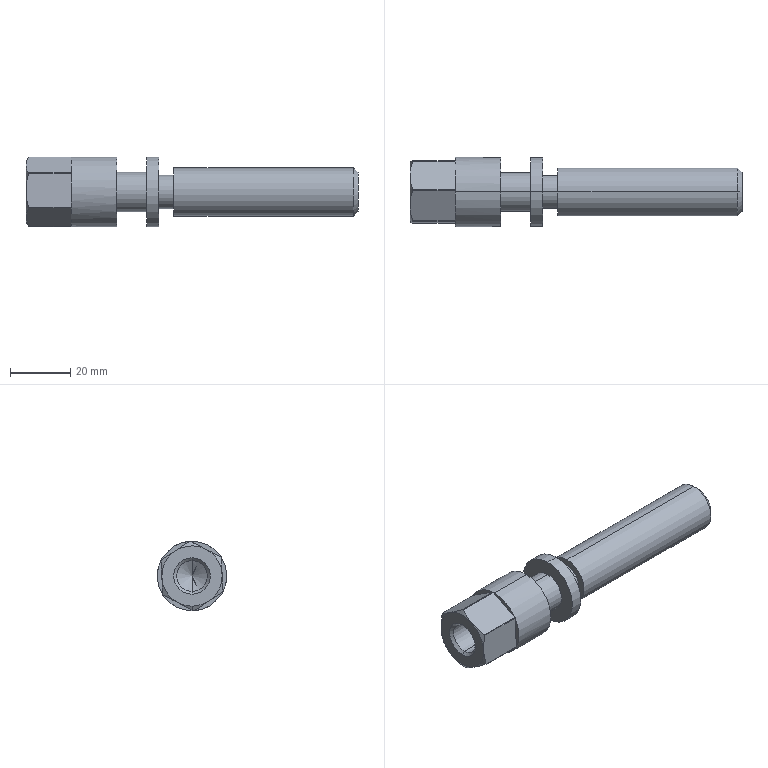Part | SolidWorks | features 3DProfileFeature 1, Chamfer 1, HoleWzd 1, ICE 1, Revolution 1 | 1 solid | 43 faces | box 110 x 23 x 23 mm | volume 25098 mm3 | plane 18 | cone 13 | cylinder 12 | commonest cylinder face diameters 23 x4 10.2 x2 11 x2 13 x2 16 x2
STEP:
#1=CARTESIAN_POINT('',(110.,0.,-6.5));
#2=VERTEX_POINT('',#1);
#3=CARTESIAN_POINT('',(110.,0.,6.5));
#4=VERTEX_POINT('',#3);
#5=CARTESIAN_POINT('',(110.,0.,0.));
#6=DIRECTION('',(1.,0.,0.));
#7=DIRECTION('',(0.,0.,1.));
#8=AXIS2_PLACEMENT_3D('',#5,#6,#7);
#9=CIRCLE('',#8,6.5);
#10=EDGE_CURVE('',#2,#4,#9,.T.);
#11=ORIENTED_EDGE('',*,*,#10,.F.);
#12=CARTESIAN_POINT('',(108.5,0.,-8.));
#13=VERTEX_POINT('',#12);
#14=CARTESIAN_POINT('',(108.5,0.,-8.));
#15=DIRECTION('',(-0.7071,0.,-0.7071));
#16=VECTOR('',#15,1000.);
#17=LINE('',#14,#16);
#18=EDGE_CURVE('',#2,#13,#17,.T.);
#19=ORIENTED_EDGE('',*,*,#18,.T.);
#20=CARTESIAN_POINT('',(108.5,0.,8.));
#21=VERTEX_POINT('',#20);
#22=CARTESIAN_POINT('',(108.5,0.,0.));
#23=DIRECTION('',(-1.,0.,0.));
#24=DIRECTION('',(0.,0.,1.));
#25=AXIS2_PLACEMENT_3D('',#22,#23,#24);
#26=CIRCLE('',#25,8.);
#27=EDGE_CURVE('',#21,#13,#26,.T.);
#28=ORIENTED_EDGE('',*,*,#27,.F.);
#29=CARTESIAN_POINT('',(108.5,0.,8.));
#30=DIRECTION('',(-0.7071,0.,0.7071));
#31=VECTOR('',#30,1000.);
#32=LINE('',#29,#31);
#33=EDGE_CURVE('',#4,#21,#32,.T.);
#34=ORIENTED_EDGE('',*,*,#33,.F.);
#35=EDGE_LOOP('',(#11,#19,#28,#34));
#36=FACE_OUTER_BOUND('',#35,.T.);
#37=CARTESIAN_POINT('',(108.5,0.,0.));
#38=DIRECTION('',(-1.,0.,0.));
#39=DIRECTION('',(0.,0.,1.));
#40=AXIS2_PLACEMENT_3D('',#37,#38,#39);
#41=CONICAL_SURFACE('',#40,8.,0.7854);
#42=ADVANCED_FACE('',(#36),#41,.T.);
#43=CARTESIAN_POINT('',(0.925,0.,-5.1));
#44=VERTEX_POINT('',#43);
#45=CARTESIAN_POINT('',(0.925,0.,5.1));
#46=VERTEX_POINT('',#45);
#47=CARTESIAN_POINT('',(0.925,0.,0.));
#48=DIRECTION('',(-1.,0.,0.));
#49=DIRECTION('',(0.,0.,1.));
#50=AXIS2_PLACEMENT_3D('',#47,#48,#49);
#51=CIRCLE('',#50,5.1);
#52=EDGE_CURVE('',#44,#46,#51,.T.);
#53=ORIENTED_EDGE('',*,*,#52,.F.);
#54=CARTESIAN_POINT('',(0.,0.,-6.025));
#55=VERTEX_POINT('',#54);
#56=CARTESIAN_POINT('',(0.,0.,-6.025));
#57=DIRECTION('',(-0.7071,0.,-0.7071));
#58=VECTOR('',#57,1000.);
#59=LINE('',#56,#58);
#60=EDGE_CURVE('',#44,#55,#59,.T.);
#61=ORIENTED_EDGE('',*,*,#60,.T.);
#62=CARTESIAN_POINT('',(0.,0.,6.025));
#63=VERTEX_POINT('',#62);
#64=CARTESIAN_POINT('',(0.,0.,0.));
#65=DIRECTION('',(-1.,0.,0.));
#66=DIRECTION('',(0.,0.,1.));
#67=AXIS2_PLACEMENT_3D('',#64,#65,#66);
#68=CIRCLE('',#67,6.025);
#69=EDGE_CURVE('',#55,#63,#68,.T.);
#70=ORIENTED_EDGE('',*,*,#69,.T.);
#71=CARTESIAN_POINT('',(0.,0.,6.025));
#72=DIRECTION('',(-0.7071,0.,0.7071));
#73=VECTOR('',#72,1000.);
#74=LINE('',#71,#73);
#75=EDGE_CURVE('',#46,#63,#74,.T.);
#76=ORIENTED_EDGE('',*,*,#75,.F.);
#77=EDGE_LOOP('',(#53,#61,#70,#76));
#78=FACE_OUTER_BOUND('',#77,.T.);
#79=CARTESIAN_POINT('',(0.,0.,0.));
#80=DIRECTION('',(-1.,0.,0.));
#81=DIRECTION('',(0.,0.,1.));
#82=AXIS2_PLACEMENT_3D('',#79,#80,#81);
#83=CONICAL_SURFACE('',#82,6.025,0.7854);
#84=ADVANCED_FACE('',(#78),#83,.F.);
#85=CARTESIAN_POINT('',(23.25,0.,-5.1));
#86=VERTEX_POINT('',#85);
#87=CARTESIAN_POINT('',(23.25,0.,5.1));
#88=VERTEX_POINT('',#87);
#89=CARTESIAN_POINT('',(23.25,0.,0.));
#90=DIRECTION('',(-1.,0.,0.));
#91=DIRECTION('',(0.,0.,1.));
#92=AXIS2_PLACEMENT_3D('',#89,#90,#91);
#93=CIRCLE('',#92,5.1);
#94=EDGE_CURVE('',#86,#88,#93,.T.);
#95=ORIENTED_EDGE('',*,*,#94,.F.);
#96=CARTESIAN_POINT('',(0.,0.,-5.1));
#97=DIRECTION('',(-1.,0.,0.));
#98=VECTOR('',#97,1000.);
#99=LINE('',#96,#98);
#100=EDGE_CURVE('',#86,#44,#99,.T.);
#101=ORIENTED_EDGE('',*,*,#100,.T.);
#102=ORIENTED_EDGE('',*,*,#52,.T.);
#103=CARTESIAN_POINT('',(0.,0.,5.1));
#104=DIRECTION('',(-1.,0.,0.));
#105=VECTOR('',#104,1000.);
#106=LINE('',#103,#105);
#107=EDGE_CURVE('',#88,#46,#106,.T.);
#108=ORIENTED_EDGE('',*,*,#107,.F.);
#109=EDGE_LOOP('',(#95,#101,#102,#108));
#110=FACE_OUTER_BOUND('',#109,.T.);
#111=CARTESIAN_POINT('',(0.,0.,0.));
#112=DIRECTION('',(-1.,0.,0.));
#113=DIRECTION('',(0.,0.,1.));
#114=AXIS2_PLACEMENT_3D('',#111,#112,#113);
#115=CYLINDRICAL_SURFACE('',#114,5.1);
#116=ADVANCED_FACE('',(#110),#115,.F.);
#117=CARTESIAN_POINT('',(26.314,0.,0.));
#118=VERTEX_POINT('',#117);
#119=CARTESIAN_POINT('',(23.25,0.,5.1));
#120=DIRECTION('',(-0.515,0.,0.8572));
#121=VECTOR('',#120,1000.);
#122=LINE('',#119,#121);
#123=EDGE_CURVE('',#118,#88,#122,.T.);
#124=ORIENTED_EDGE('',*,*,#123,.F.);
#125=CARTESIAN_POINT('',(23.25,0.,-5.1));
#126=DIRECTION('',(-0.515,0.,-0.8572));
#127=VECTOR('',#126,1000.);
#128=LINE('',#125,#127);
#129=EDGE_CURVE('',#118,#86,#128,.T.);
#130=ORIENTED_EDGE('',*,*,#129,.T.);
#131=ORIENTED_EDGE('',*,*,#94,.T.);
#132=EDGE_LOOP('',(#124,#130,#131));
#133=FACE_OUTER_BOUND('',#132,.T.);
#134=CARTESIAN_POINT('',(23.25,0.,0.));
#135=DIRECTION('',(-1.,0.,0.));
#136=DIRECTION('',(0.,0.,1.));
#137=AXIS2_PLACEMENT_3D('',#134,#135,#136);
#138=CONICAL_SURFACE('',#137,5.1,1.03);
#139=ADVANCED_FACE('',(#133),#138,.F.);
#140=ORIENTED_EDGE('',*,*,#27,.T.);
#141=CARTESIAN_POINT('',(49.,0.,-8.));
#142=VERTEX_POINT('',#141);
#143=CARTESIAN_POINT('',(0.,0.,-8.));
#144=DIRECTION('',(-1.,0.,0.));
#145=VECTOR('',#144,1000.);
#146=LINE('',#143,#145);
#147=EDGE_CURVE('',#13,#142,#146,.T.);
#148=ORIENTED_EDGE('',*,*,#147,.T.);
#149=CARTESIAN_POINT('',(49.,0.,8.));
#150=VERTEX_POINT('',#149);
#151=CARTESIAN_POINT('',(49.,0.,0.));
#152=DIRECTION('',(-1.,0.,0.));
#153=DIRECTION('',(0.,0.,1.));
#154=AXIS2_PLACEMENT_3D('',#151,#152,#153);
#155=CIRCLE('',#154,8.);
#156=EDGE_CURVE('',#150,#142,#155,.T.);
#157=ORIENTED_EDGE('',*,*,#156,.F.);
#158=CARTESIAN_POINT('',(0.,0.,8.));
#159=DIRECTION('',(-1.,0.,0.));
#160=VECTOR('',#159,1000.);
#161=LINE('',#158,#160);
#162=EDGE_CURVE('',#21,#150,#161,.T.);
#163=ORIENTED_EDGE('',*,*,#162,.F.);
#164=EDGE_LOOP('',(#140,#148,#157,#163));
#165=FACE_OUTER_BOUND('',#164,.T.);
#166=CARTESIAN_POINT('',(0.,0.,0.));
#167=DIRECTION('',(-1.,0.,0.));
#168=DIRECTION('',(0.,0.,1.));
#169=AXIS2_PLACEMENT_3D('',#166,#167,#168);
#170=CYLINDRICAL_SURFACE('',#169,8.);
#171=ADVANCED_FACE('',(#165),#170,.T.);
#172=CARTESIAN_POINT('',(49.,0.,5.5));
#173=VERTEX_POINT('',#172);
#174=CARTESIAN_POINT('',(49.,0.,-5.5));
#175=VERTEX_POINT('',#174);
#176=CARTESIAN_POINT('',(49.,0.,0.));
#177=DIRECTION('',(-1.,0.,0.));
#178=DIRECTION('',(0.,0.,1.));
#179=AXIS2_PLACEMENT_3D('',#176,#177,#178);
#180=CIRCLE('',#179,5.5);
#181=EDGE_CURVE('',#173,#175,#180,.T.);
#182=ORIENTED_EDGE('',*,*,#181,.T.);
#183=CARTESIAN_POINT('',(44.,0.,-5.5));
#184=VERTEX_POINT('',#183);
#185=CARTESIAN_POINT('',(0.,0.,-5.5));
#186=DIRECTION('',(-1.,0.,0.));
#187=VECTOR('',#186,1000.);
#188=LINE('',#185,#187);
#189=EDGE_CURVE('',#175,#184,#188,.T.);
#190=ORIENTED_EDGE('',*,*,#189,.T.);
#191=CARTESIAN_POINT('',(44.,0.,5.5));
#192=VERTEX_POINT('',#191);
#193=CARTESIAN_POINT('',(44.,0.,0.));
#194=DIRECTION('',(-1.,0.,0.));
#195=DIRECTION('',(0.,0.,1.));
#196=AXIS2_PLACEMENT_3D('',#193,#194,#195);
#197=CIRCLE('',#196,5.5);
#198=EDGE_CURVE('',#192,#184,#197,.T.);
#199=ORIENTED_EDGE('',*,*,#198,.F.);
#200=CARTESIAN_POINT('',(0.,0.,5.5));
#201=DIRECTION('',(-1.,0.,0.));
#202=VECTOR('',#201,1000.);
#203=LINE('',#200,#202);
#204=EDGE_CURVE('',#173,#192,#203,.T.);
#205=ORIENTED_EDGE('',*,*,#204,.F.);
#206=EDGE_LOOP('',(#182,#190,#199,#205));
#207=FACE_OUTER_BOUND('',#206,.T.);
#208=CARTESIAN_POINT('',(0.,0.,0.));
#209=DIRECTION('',(-1.,0.,0.));
#210=DIRECTION('',(0.,0.,1.));
#211=AXIS2_PLACEMENT_3D('',#208,#209,#210);
#212=CYLINDRICAL_SURFACE('',#211,5.5);
#213=ADVANCED_FACE('',(#207),#212,.T.);
#214=CARTESIAN_POINT('',(44.,0.,11.5));
#215=VERTEX_POINT('',#214);
#216=CARTESIAN_POINT('',(44.,0.,-11.5));
#217=VERTEX_POINT('',#216);
#218=CARTESIAN_POINT('',(44.,0.,0.));
#219=DIRECTION('',(-1.,0.,0.));
#220=DIRECTION('',(0.,0.,1.));
#221=AXIS2_PLACEMENT_3D('',#218,#219,#220);
#222=CIRCLE('',#221,11.5);
#223=EDGE_CURVE('',#215,#217,#222,.T.);
#224=ORIENTED_EDGE('',*,*,#223,.T.);
#225=CARTESIAN_POINT('',(40.,0.,-11.5));
#226=VERTEX_POINT('',#225);
#227=CARTESIAN_POINT('',(0.,0.,-11.5));
#228=DIRECTION('',(-1.,0.,0.));
#229=VECTOR('',#228,1000.);
#230=LINE('',#227,#229);
#231=EDGE_CURVE('',#217,#226,#230,.T.);
#232=ORIENTED_EDGE('',*,*,#231,.T.);
#233=CARTESIAN_POINT('',(40.,0.,11.5));
#234=VERTEX_POINT('',#233);
#235=CARTESIAN_POINT('',(40.,0.,0.));
#236=DIRECTION('',(-1.,0.,0.));
#237=DIRECTION('',(0.,0.,1.));
#238=AXIS2_PLACEMENT_3D('',#235,#236,#237);
#239=CIRCLE('',#238,11.5);
#240=EDGE_CURVE('',#234,#226,#239,.T.);
#241=ORIENTED_EDGE('',*,*,#240,.F.);
#242=CARTESIAN_POINT('',(0.,0.,11.5));
#243=DIRECTION('',(-1.,0.,0.));
#244=VECTOR('',#243,1000.);
#245=LINE('',#242,#244);
#246=EDGE_CURVE('',#215,#234,#245,.T.);
#247=ORIENTED_EDGE('',*,*,#246,.F.);
#248=EDGE_LOOP('',(#224,#232,#241,#247));
#249=FACE_OUTER_BOUND('',#248,.T.);
#250=CARTESIAN_POINT('',(0.,0.,0.));
#251=DIRECTION('',(-1.,0.,0.));
#252=DIRECTION('',(0.,0.,1.));
#253=AXIS2_PLACEMENT_3D('',#250,#251,#252);
#254=CYLINDRICAL_SURFACE('',#253,11.5);
#255=ADVANCED_FACE('',(#249),#254,.T.);
#256=CARTESIAN_POINT('',(40.,0.,6.5));
#257=VERTEX_POINT('',#256);
#258=CARTESIAN_POINT('',(40.,0.,-6.5));
#259=VERTEX_POINT('',#258);
#260=CARTESIAN_POINT('',(40.,0.,0.));
#261=DIRECTION('',(-1.,0.,0.));
#262=DIRECTION('',(0.,0.,1.));
#263=AXIS2_PLACEMENT_3D('',#260,#261,#262);
#264=CIRCLE('',#263,6.5);
#265=EDGE_CURVE('',#257,#259,#264,.T.);
#266=ORIENTED_EDGE('',*,*,#265,.T.);
#267=CARTESIAN_POINT('',(30.,0.,-6.5));
#268=VERTEX_POINT('',#267);
#269=CARTESIAN_POINT('',(0.,0.,-6.5));
#270=DIRECTION('',(-1.,0.,0.));
#271=VECTOR('',#270,1000.);
#272=LINE('',#269,#271);
#273=EDGE_CURVE('',#259,#268,#272,.T.);
#274=ORIENTED_EDGE('',*,*,#273,.T.);
#275=CARTESIAN_POINT('',(30.,0.,6.5));
#276=VERTEX_POINT('',#275);
#277=CARTESIAN_POINT('',(30.,0.,0.));
#278=DIRECTION('',(-1.,0.,0.));
#279=DIRECTION('',(0.,0.,1.));
#280=AXIS2_PLACEMENT_3D('',#277,#278,#279);
#281=CIRCLE('',#280,6.5);
#282=EDGE_CURVE('',#276,#268,#281,.T.);
#283=ORIENTED_EDGE('',*,*,#282,.F.);
#284=CARTESIAN_POINT('',(0.,0.,6.5));
#285=DIRECTION('',(-1.,0.,0.));
#286=VECTOR('',#285,1000.);
#287=LINE('',#284,#286);
#288=EDGE_CURVE('',#257,#276,#287,.T.);
#289=ORIENTED_EDGE('',*,*,#288,.F.);
#290=EDGE_LOOP('',(#266,#274,#283,#289));
#291=FACE_OUTER_BOUND('',#290,.T.);
#292=CARTESIAN_POINT('',(0.,0.,0.));
#293=DIRECTION('',(-1.,0.,0.));
#294=DIRECTION('',(0.,0.,1.));
#295=AXIS2_PLACEMENT_3D('',#292,#293,#294);
#296=CYLINDRICAL_SURFACE('',#295,6.5);
#297=ADVANCED_FACE('',(#291),#296,.T.);
#298=CARTESIAN_POINT('',(30.,0.,11.5));
#299=VERTEX_POINT('',#298);
#300=CARTESIAN_POINT('',(30.,0.,-11.5));
#301=VERTEX_POINT('',#300);
#302=CARTESIAN_POINT('',(30.,0.,0.));
#303=DIRECTION('',(-1.,0.,0.));
#304=DIRECTION('',(0.,0.,1.));
#305=AXIS2_PLACEMENT_3D('',#302,#303,#304);
#306=CIRCLE('',#305,11.5);
#307=EDGE_CURVE('',#299,#301,#306,.T.);
#308=ORIENTED_EDGE('',*,*,#307,.T.);
#309=CARTESIAN_POINT('',(15.,0.,-11.5));
#310=VERTEX_POINT('',#309);
#311=CARTESIAN_POINT('',(0.,0.,-11.5));
#312=DIRECTION('',(-1.,0.,0.));
#313=VECTOR('',#312,1000.);
#314=LINE('',#311,#313);
#315=EDGE_CURVE('',#301,#310,#314,.T.);
#316=ORIENTED_EDGE('',*,*,#315,.T.);
#317=CARTESIAN_POINT('',(15.,9.591,-6.346));
#318=VERTEX_POINT('',#317);
#319=CARTESIAN_POINT('',(15.,0.,0.));
#320=DIRECTION('',(-1.,0.,0.));
#321=DIRECTION('',(0.,0.,1.));
#322=AXIS2_PLACEMENT_3D('',#319,#320,#321);
#323=CIRCLE('',#322,11.5);
#324=EDGE_CURVE('',#318,#310,#323,.T.);
#325=ORIENTED_EDGE('',*,*,#324,.F.);
#326=CARTESIAN_POINT('',(0.866,9.591,-6.346));
#327=VERTEX_POINT('',#326);
#328=CARTESIAN_POINT('',(0.,9.591,-6.346));
#329=DIRECTION('',(1.,0.,0.));
#330=VECTOR('',#329,1000.);
#331=LINE('',#328,#330);
#332=EDGE_CURVE('',#327,#318,#331,.T.);
#333=ORIENTED_EDGE('',*,*,#332,.F.);
#334=CARTESIAN_POINT('',(0.866,9.68,-6.208));
#335=VERTEX_POINT('',#334);
#336=CARTESIAN_POINT('',(0.866,0.,0.));
#337=DIRECTION('',(-1.,0.,0.));
#338=DIRECTION('',(0.,0.,1.));
#339=AXIS2_PLACEMENT_3D('',#336,#337,#338);
#340=CIRCLE('',#339,11.5);
#341=EDGE_CURVE('',#335,#327,#340,.T.);
#342=ORIENTED_EDGE('',*,*,#341,.F.);
#343=CARTESIAN_POINT('',(15.,9.68,-6.208));
#344=VERTEX_POINT('',#343);
#345=CARTESIAN_POINT('',(0.,9.68,-6.208));
#346=DIRECTION('',(-1.,0.,0.));
#347=VECTOR('',#346,1000.);
#348=LINE('',#345,#347);
#349=EDGE_CURVE('',#344,#335,#348,.T.);
#350=ORIENTED_EDGE('',*,*,#349,.F.);
#351=CARTESIAN_POINT('',(15.,10.291,5.133));
#352=VERTEX_POINT('',#351);
#353=CARTESIAN_POINT('',(15.,0.,0.));
#354=DIRECTION('',(-1.,0.,0.));
#355=DIRECTION('',(0.,0.,1.));
#356=AXIS2_PLACEMENT_3D('',#353,#354,#355);
#357=CIRCLE('',#356,11.5);
#358=EDGE_CURVE('',#352,#344,#357,.T.);
#359=ORIENTED_EDGE('',*,*,#358,.F.);
#360=CARTESIAN_POINT('',(0.866,10.291,5.133));
#361=VERTEX_POINT('',#360);
#362=CARTESIAN_POINT('',(0.,10.291,5.133));
#363=DIRECTION('',(1.,0.,0.));
#364=VECTOR('',#363,1000.);
#365=LINE('',#362,#364);
#366=EDGE_CURVE('',#361,#352,#365,.T.);
#367=ORIENTED_EDGE('',*,*,#366,.F.);
#368=CARTESIAN_POINT('',(0.866,10.217,5.279));
#369=VERTEX_POINT('',#368);
#370=CARTESIAN_POINT('',(0.866,0.,0.));
#371=DIRECTION('',(-1.,0.,0.));
#372=DIRECTION('',(0.,0.,1.));
#373=AXIS2_PLACEMENT_3D('',#370,#371,#372);
#374=CIRCLE('',#373,11.5);
#375=EDGE_CURVE('',#369,#361,#374,.T.);
#376=ORIENTED_EDGE('',*,*,#375,.F.);
#377=CARTESIAN_POINT('',(15.,10.217,5.279));
#378=VERTEX_POINT('',#377);
#379=CARTESIAN_POINT('',(0.,10.217,5.279));
#380=DIRECTION('',(-1.,0.,0.));
#381=VECTOR('',#380,1000.);
#382=LINE('',#379,#381);
#383=EDGE_CURVE('',#378,#369,#382,.T.);
#384=ORIENTED_EDGE('',*,*,#383,.F.);
#385=CARTESIAN_POINT('',(15.,0.7003,11.479));
#386=VERTEX_POINT('',#385);
#387=CARTESIAN_POINT('',(15.,0.,0.));
#388=DIRECTION('',(-1.,0.,0.));
#389=DIRECTION('',(0.,0.,1.));
#390=AXIS2_PLACEMENT_3D('',#387,#388,#389);
#391=CIRCLE('',#390,11.5);
#392=EDGE_CURVE('',#386,#378,#391,.T.);
#393=ORIENTED_EDGE('',*,*,#392,.F.);
#394=CARTESIAN_POINT('',(0.866,0.7003,11.479));
#395=VERTEX_POINT('',#394);
#396=CARTESIAN_POINT('',(0.,0.7003,11.479));
#397=DIRECTION('',(1.,0.,0.));
#398=VECTOR('',#397,1000.);
#399=LINE('',#396,#398);
#400=EDGE_CURVE('',#395,#386,#399,.T.);
#401=ORIENTED_EDGE('',*,*,#400,.F.);
#402=CARTESIAN_POINT('',(0.866,0.5366,11.487));
#403=VERTEX_POINT('',#402);
#404=CARTESIAN_POINT('',(0.866,0.,0.));
#405=DIRECTION('',(-1.,0.,0.));
#406=DIRECTION('',(0.,0.,1.));
#407=AXIS2_PLACEMENT_3D('',#404,#405,#406);
#408=CIRCLE('',#407,11.5);
#409=EDGE_CURVE('',#403,#395,#408,.T.);
#410=ORIENTED_EDGE('',*,*,#409,.F.);
#411=CARTESIAN_POINT('',(15.,0.5366,11.487));
#412=VERTEX_POINT('',#411);
#413=CARTESIAN_POINT('',(0.,0.5366,11.487));
#414=DIRECTION('',(-1.,0.,0.));
#415=VECTOR('',#414,1000.);
#416=LINE('',#413,#415);
#417=EDGE_CURVE('',#412,#403,#416,.T.);
#418=ORIENTED_EDGE('',*,*,#417,.F.);
#419=CARTESIAN_POINT('',(15.,0.,11.5));
#420=VERTEX_POINT('',#419);
#421=CARTESIAN_POINT('',(15.,0.,0.));
#422=DIRECTION('',(-1.,0.,0.));
#423=DIRECTION('',(0.,0.,1.));
#424=AXIS2_PLACEMENT_3D('',#421,#422,#423);
#425=CIRCLE('',#424,11.5);
#426=EDGE_CURVE('',#420,#412,#425,.T.);
#427=ORIENTED_EDGE('',*,*,#426,.F.);
#428=CARTESIAN_POINT('',(0.,0.,11.5));
#429=DIRECTION('',(-1.,0.,0.));
#430=VECTOR('',#429,1000.);
#431=LINE('',#428,#430);
#432=EDGE_CURVE('',#299,#420,#431,.T.);
#433=ORIENTED_EDGE('',*,*,#432,.F.);
#434=EDGE_LOOP('',(#308,#316,#325,#333,#342,#350,#359,#367,#376,#384,#393,#401,#410,#418,#427,#433));
#435=FACE_OUTER_BOUND('',#434,.T.);
#436=CARTESIAN_POINT('',(0.,0.,0.));
#437=DIRECTION('',(-1.,0.,0.));
#438=DIRECTION('',(0.,0.,1.));
#439=AXIS2_PLACEMENT_3D('',#436,#437,#438);
#440=CYLINDRICAL_SURFACE('',#439,11.5);
#441=ADVANCED_FACE('',(#435),#440,.T.);
#442=CARTESIAN_POINT('',(0.,0.,-10.));
#443=VERTEX_POINT('',#442);
#444=CARTESIAN_POINT('',(0.,-5.459,-8.379));
#445=VERTEX_POINT('',#444);
#446=CARTESIAN_POINT('',(0.,0.,0.));
#447=DIRECTION('',(-1.,0.,0.));
#448=DIRECTION('',(0.,0.,1.));
#449=AXIS2_PLACEMENT_3D('',#446,#447,#448);
#450=CIRCLE('',#449,10.);
#451=EDGE_CURVE('',#443,#445,#450,.T.);
#452=ORIENTED_EDGE('',*,*,#451,.F.);
#453=CARTESIAN_POINT('',(0.7015,0.,-11.215));
#454=VERTEX_POINT('',#453);
#455=CARTESIAN_POINT('',(0.866,0.,-11.5));
#456=DIRECTION('',(0.5,0.,-0.866));
#457=VECTOR('',#456,1000.);
#458=LINE('',#455,#457);
#459=EDGE_CURVE('',#443,#454,#458,.T.);
#460=ORIENTED_EDGE('',*,*,#459,.T.);
#461=CARTESIAN_POINT('',(0.866,-0.5366,-11.487));
#462=VERTEX_POINT('',#461);
#463=CARTESIAN_POINT('',(0.866,-0.5366,-11.487));
#464=CARTESIAN_POINT('',(0.8089,-0.358,-11.397));
#465=CARTESIAN_POINT('',(0.754,-0.1792,-11.306));
#466=CARTESIAN_POINT('',(0.7015,0.,-11.215));
#467=B_SPLINE_CURVE_WITH_KNOTS('',3,(#463,#464,#465,#466),.UNSPECIFIED.,.F.,.F.,(4,4),(0.000000722,0.0006195),.UNSPECIFIED.);
#468=EDGE_CURVE('',#462,#454,#467,.T.);
#469=ORIENTED_EDGE('',*,*,#468,.F.);
#470=CARTESIAN_POINT('',(0.866,-0.7003,-11.479));
#471=VERTEX_POINT('',#470);
#472=CARTESIAN_POINT('',(0.866,0.,0.));
#473=DIRECTION('',(-1.,0.,0.));
#474=DIRECTION('',(0.,0.,1.));
#475=AXIS2_PLACEMENT_3D('',#472,#473,#474);
#476=CIRCLE('',#475,11.5);
#477=EDGE_CURVE('',#462,#471,#476,.T.);
#478=ORIENTED_EDGE('',*,*,#477,.T.);
#479=CARTESIAN_POINT('',(0.,-5.459,-8.379));
#480=CARTESIAN_POINT('',(0.,-5.055,-8.642));
#481=CARTESIAN_POINT('',(0.02038,-4.65,-8.906));
#482=CARTESIAN_POINT('',(0.0994,-3.847,-9.428));
#483=CARTESIAN_POINT('',(0.158,-3.449,-9.688));
#484=CARTESIAN_POINT('',(0.384,-2.26,-10.462));
#485=CARTESIAN_POINT('',(0.6017,-1.477,-10.973));
#486=CARTESIAN_POINT('',(0.866,-0.7003,-11.479));
#487=B_SPLINE_CURVE_WITH_KNOTS('',3,(#479,#480,#481,#482,#483,#484,#485,#486),.UNSPECIFIED.,.F.,.F.,(4,2,2,4),(0.005745,0.007175,0.008605,0.01146),.UNSPECIFIED.);
#488=EDGE_CURVE('',#445,#471,#487,.T.);
#489=ORIENTED_EDGE('',*,*,#488,.F.);
#490=EDGE_LOOP('',(#452,#460,#469,#478,#489));
#491=FACE_OUTER_BOUND('',#490,.T.);
#492=CARTESIAN_POINT('',(0.866,0.,0.));
#493=DIRECTION('',(1.,0.,0.));
#494=DIRECTION('',(0.,0.,-1.));
#495=AXIS2_PLACEMENT_3D('',#492,#493,#494);
#496=CONICAL_SURFACE('',#495,11.5,1.047);
#497=ADVANCED_FACE('',(#491),#496,.T.);
#498=CARTESIAN_POINT('',(0.,5.459,8.379));
#499=VERTEX_POINT('',#498);
#500=CARTESIAN_POINT('',(0.866,10.217,5.279));
#501=CARTESIAN_POINT('',(0.601,9.438,5.786));
#502=CARTESIAN_POINT('',(0.3831,8.653,6.297));
#503=CARTESIAN_POINT('',(0.08218,7.069,7.33));
#504=CARTESIAN_POINT('',(0.,6.268,7.851));
#505=CARTESIAN_POINT('',(0.,5.459,8.379));
#506=B_SPLINE_CURVE_WITH_KNOTS('',3,(#500,#501,#502,#503,#504,#505),.UNSPECIFIED.,.F.,.F.,(4,2,4),(0.000000722,0.002873,0.005745),.UNSPECIFIED.);
#507=EDGE_CURVE('',#369,#499,#506,.T.);
#508=ORIENTED_EDGE('',*,*,#507,.F.);
#509=ORIENTED_EDGE('',*,*,#375,.T.);
#510=CARTESIAN_POINT('',(0.,9.986,-0.5378));
#511=VERTEX_POINT('',#510);
#512=CARTESIAN_POINT('',(0.,9.986,-0.5378));
#513=CARTESIAN_POINT('',(0.,10.011,-0.05725));
#514=CARTESIAN_POINT('',(0.02038,10.037,0.4261));
#515=CARTESIAN_POINT('',(0.0994,10.089,1.382));
#516=CARTESIAN_POINT('',(0.158,10.115,1.857));
#517=CARTESIAN_POINT('',(0.384,10.191,3.274));
#518=CARTESIAN_POINT('',(0.6017,10.241,4.207));
#519=CARTESIAN_POINT('',(0.866,10.291,5.133));
#520=B_SPLINE_CURVE_WITH_KNOTS('',3,(#512,#513,#514,#515,#516,#517,#518,#519),.UNSPECIFIED.,.F.,.F.,(4,2,2,4),(0.005745,0.007175,0.008605,0.01146),.UNSPECIFIED.);
#521=EDGE_CURVE('',#511,#361,#520,.T.);
#522=ORIENTED_EDGE('',*,*,#521,.F.);
#523=CARTESIAN_POINT('',(0.,0.,0.));
#524=DIRECTION('',(-1.,0.,0.));
#525=DIRECTION('',(0.,0.,1.));
#526=AXIS2_PLACEMENT_3D('',#523,#524,#525);
#527=CIRCLE('',#526,10.);
#528=EDGE_CURVE('',#499,#511,#527,.T.);
#529=ORIENTED_EDGE('',*,*,#528,.F.);
#530=EDGE_LOOP('',(#508,#509,#522,#529));
#531=FACE_OUTER_BOUND('',#530,.T.);
#532=CARTESIAN_POINT('',(0.866,0.,0.));
#533=DIRECTION('',(1.,0.,0.));
#534=DIRECTION('',(0.,0.,-1.));
#535=AXIS2_PLACEMENT_3D('',#532,#533,#534);
#536=CONICAL_SURFACE('',#535,11.5,1.047);
#537=ADVANCED_FACE('',(#531),#536,.T.);
#538=CARTESIAN_POINT('',(0.,5.459,8.379));
#539=CARTESIAN_POINT('',(0.,5.055,8.642));
#540=CARTESIAN_POINT('',(0.02038,4.65,8.906));
#541=CARTESIAN_POINT('',(0.0994,3.847,9.428));
#542=CARTESIAN_POINT('',(0.158,3.449,9.688));
#543=CARTESIAN_POINT('',(0.384,2.26,10.462));
#544=CARTESIAN_POINT('',(0.6017,1.477,10.973));
#545=CARTESIAN_POINT('',(0.866,0.7003,11.479));
#546=B_SPLINE_CURVE_WITH_KNOTS('',3,(#538,#539,#540,#541,#542,#543,#544,#545),.UNSPECIFIED.,.F.,.F.,(4,2,2,4),(0.005745,0.007175,0.008605,0.01146),.UNSPECIFIED.);
#547=EDGE_CURVE('',#499,#395,#546,.T.);
#548=ORIENTED_EDGE('',*,*,#547,.F.);
#549=CARTESIAN_POINT('',(0.,-4.527,8.917));
#550=VERTEX_POINT('',#549);
#551=CARTESIAN_POINT('',(0.,0.,0.));
#552=DIRECTION('',(-1.,0.,0.));
#553=DIRECTION('',(0.,0.,1.));
#554=AXIS2_PLACEMENT_3D('',#551,#552,#553);
#555=CIRCLE('',#554,10.);
#556=EDGE_CURVE('',#550,#499,#555,.T.);
#557=ORIENTED_EDGE('',*,*,#556,.F.);
#558=CARTESIAN_POINT('',(0.866,0.5366,11.487));
#559=CARTESIAN_POINT('',(0.601,-0.2923,11.067));
#560=CARTESIAN_POINT('',(0.3831,-1.127,10.643));
#561=CARTESIAN_POINT('',(0.08218,-2.813,9.787));
#562=CARTESIAN_POINT('',(0.,-3.665,9.354));
#563=CARTESIAN_POINT('',(0.,-4.527,8.917));
#564=B_SPLINE_CURVE_WITH_KNOTS('',3,(#558,#559,#560,#561,#562,#563),.UNSPECIFIED.,.F.,.F.,(4,2,4),(0.000000722,0.002873,0.005745),.UNSPECIFIED.);
#565=EDGE_CURVE('',#403,#550,#564,.T.);
#566=ORIENTED_EDGE('',*,*,#565,.F.);
#567=ORIENTED_EDGE('',*,*,#409,.T.);
#568=EDGE_LOOP('',(#548,#557,#566,#567));
#569=FACE_OUTER_BOUND('',#568,.T.);
#570=CARTESIAN_POINT('',(0.866,0.,0.));
#571=DIRECTION('',(1.,0.,0.));
#572=DIRECTION('',(0.,0.,-1.));
#573=AXIS2_PLACEMENT_3D('',#570,#571,#572);
#574=CONICAL_SURFACE('',#573,11.5,1.047);
#575=ADVANCED_FACE('',(#569),#574,.T.);
#576=CARTESIAN_POINT('',(0.866,-9.591,6.346));
#577=VERTEX_POINT('',#576);
#578=CARTESIAN_POINT('',(0.,-4.527,8.917));
#579=CARTESIAN_POINT('',(0.,-4.956,8.699));
#580=CARTESIAN_POINT('',(0.02038,-5.388,8.48));
#581=CARTESIAN_POINT('',(0.0994,-6.242,8.046));
#582=CARTESIAN_POINT('',(0.158,-6.666,7.831));
#583=CARTESIAN_POINT('',(0.384,-7.931,7.189));
#584=CARTESIAN_POINT('',(0.6017,-8.764,6.765));
#585=CARTESIAN_POINT('',(0.866,-9.591,6.346));
#586=B_SPLINE_CURVE_WITH_KNOTS('',3,(#578,#579,#580,#581,#582,#583,#584,#585),.UNSPECIFIED.,.F.,.F.,(4,2,2,4),(0.005745,0.007175,0.008605,0.01146),.UNSPECIFIED.);
#587=EDGE_CURVE('',#550,#577,#586,.T.);
#588=ORIENTED_EDGE('',*,*,#587,.F.);
#589=CARTESIAN_POINT('',(0.,-9.986,0.5378));
#590=VERTEX_POINT('',#589);
#591=CARTESIAN_POINT('',(0.,0.,0.));
#592=DIRECTION('',(-1.,0.,0.));
#593=DIRECTION('',(0.,0.,1.));
#594=AXIS2_PLACEMENT_3D('',#591,#592,#593);
#595=CIRCLE('',#594,10.);
#596=EDGE_CURVE('',#590,#550,#595,.T.);
#597=ORIENTED_EDGE('',*,*,#596,.F.);
#598=CARTESIAN_POINT('',(0.866,-9.68,6.208));
#599=VERTEX_POINT('',#598);
#600=CARTESIAN_POINT('',(0.866,-9.68,6.208));
#601=CARTESIAN_POINT('',(0.601,-9.73,5.28));
#602=CARTESIAN_POINT('',(0.3831,-9.78,4.345));
#603=CARTESIAN_POINT('',(0.08218,-9.882,2.457));
#604=CARTESIAN_POINT('',(0.,-9.934,1.503));
#605=CARTESIAN_POINT('',(0.,-9.986,0.5378));
#606=B_SPLINE_CURVE_WITH_KNOTS('',3,(#600,#601,#602,#603,#604,#605),.UNSPECIFIED.,.F.,.F.,(4,2,4),(0.000000722,0.002873,0.005745),.UNSPECIFIED.);
#607=EDGE_CURVE('',#599,#590,#606,.T.);
#608=ORIENTED_EDGE('',*,*,#607,.F.);
#609=CARTESIAN_POINT('',(0.866,0.,0.));
#610=DIRECTION('',(-1.,0.,0.));
#611=DIRECTION('',(0.,0.,1.));
#612=AXIS2_PLACEMENT_3D('',#609,#610,#611);
#613=CIRCLE('',#612,11.5);
#614=EDGE_CURVE('',#599,#577,#613,.T.);
#615=ORIENTED_EDGE('',*,*,#614,.T.);
#616=EDGE_LOOP('',(#588,#597,#608,#615));
#617=FACE_OUTER_BOUND('',#616,.T.);
#618=CARTESIAN_POINT('',(0.866,0.,0.));
#619=DIRECTION('',(1.,0.,0.));
#620=DIRECTION('',(0.,0.,-1.));
#621=AXIS2_PLACEMENT_3D('',#618,#619,#620);
#622=CONICAL_SURFACE('',#621,11.5,1.047);
#623=ADVANCED_FACE('',(#617),#622,.T.);
#624=CARTESIAN_POINT('',(0.866,-10.291,-5.133));
#625=VERTEX_POINT('',#624);
#626=CARTESIAN_POINT('',(0.,-9.986,0.5378));
#627=CARTESIAN_POINT('',(0.,-10.011,0.05725));
#628=CARTESIAN_POINT('',(0.02038,-10.037,-0.4261));
#629=CARTESIAN_POINT('',(0.0994,-10.089,-1.382));
#630=CARTESIAN_POINT('',(0.158,-10.115,-1.857));
#631=CARTESIAN_POINT('',(0.384,-10.191,-3.274));
#632=CARTESIAN_POINT('',(0.6017,-10.241,-4.207));
#633=CARTESIAN_POINT('',(0.866,-10.291,-5.133));
#634=B_SPLINE_CURVE_WITH_KNOTS('',3,(#626,#627,#628,#629,#630,#631,#632,#633),.UNSPECIFIED.,.F.,.F.,(4,2,2,4),(0.005745,0.007175,0.008605,0.01146),.UNSPECIFIED.);
#635=EDGE_CURVE('',#590,#625,#634,.T.);
#636=ORIENTED_EDGE('',*,*,#635,.F.);
#637=CARTESIAN_POINT('',(0.,0.,0.));
#638=DIRECTION('',(-1.,0.,0.));
#639=DIRECTION('',(0.,0.,1.));
#640=AXIS2_PLACEMENT_3D('',#637,#638,#639);
#641=CIRCLE('',#640,10.);
#642=EDGE_CURVE('',#445,#590,#641,.T.);
#643=ORIENTED_EDGE('',*,*,#642,.F.);
#644=CARTESIAN_POINT('',(0.866,-10.217,-5.279));
#645=VERTEX_POINT('',#644);
#646=CARTESIAN_POINT('',(0.866,-10.217,-5.279));
#647=CARTESIAN_POINT('',(0.601,-9.438,-5.786));
#648=CARTESIAN_POINT('',(0.3831,-8.653,-6.297));
#649=CARTESIAN_POINT('',(0.08218,-7.069,-7.33));
#650=CARTESIAN_POINT('',(0.,-6.268,-7.851));
#651=CARTESIAN_POINT('',(0.,-5.459,-8.379));
#652=B_SPLINE_CURVE_WITH_KNOTS('',3,(#646,#647,#648,#649,#650,#651),.UNSPECIFIED.,.F.,.F.,(4,2,4),(0.000000722,0.002873,0.005745),.UNSPECIFIED.);
#653=EDGE_CURVE('',#645,#445,#652,.T.);
#654=ORIENTED_EDGE('',*,*,#653,.F.);
#655=CARTESIAN_POINT('',(0.866,0.,0.));
#656=DIRECTION('',(-1.,0.,0.));
#657=DIRECTION('',(0.,0.,1.));
#658=AXIS2_PLACEMENT_3D('',#655,#656,#657);
#659=CIRCLE('',#658,11.5);
#660=EDGE_CURVE('',#645,#625,#659,.T.);
#661=ORIENTED_EDGE('',*,*,#660,.T.);
#662=EDGE_LOOP('',(#636,#643,#654,#661));
#663=FACE_OUTER_BOUND('',#662,.T.);
#664=CARTESIAN_POINT('',(0.866,0.,0.));
#665=DIRECTION('',(1.,0.,0.));
#666=DIRECTION('',(0.,0.,-1.));
#667=AXIS2_PLACEMENT_3D('',#664,#665,#666);
#668=CONICAL_SURFACE('',#667,11.5,1.047);
#669=ADVANCED_FACE('',(#663),#668,.T.);
#670=ORIENTED_EDGE('',*,*,#459,.F.);
#671=CARTESIAN_POINT('',(0.,4.527,-8.917));
#672=VERTEX_POINT('',#671);
#673=CARTESIAN_POINT('',(0.,0.,0.));
#674=DIRECTION('',(-1.,0.,0.));
#675=DIRECTION('',(0.,0.,1.));
#676=AXIS2_PLACEMENT_3D('',#673,#674,#675);
#677=CIRCLE('',#676,10.);
#678=EDGE_CURVE('',#672,#443,#677,.T.);
#679=ORIENTED_EDGE('',*,*,#678,.F.);
#680=CARTESIAN_POINT('',(0.7015,0.,-11.215));
#681=CARTESIAN_POINT('',(0.484,0.742,-10.838));
#682=CARTESIAN_POINT('',(0.3075,1.489,-10.459));
#683=CARTESIAN_POINT('',(0.06525,2.997,-9.693));
#684=CARTESIAN_POINT('',(0.,3.758,-9.307));
#685=CARTESIAN_POINT('',(0.,4.527,-8.917));
#686=B_SPLINE_CURVE_WITH_KNOTS('',3,(#680,#681,#682,#683,#684,#685),.UNSPECIFIED.,.F.,.F.,(4,2,4),(0.0006195,0.003182,0.005745),.UNSPECIFIED.);
#687=EDGE_CURVE('',#454,#672,#686,.T.);
#688=ORIENTED_EDGE('',*,*,#687,.F.);
#689=EDGE_LOOP('',(#670,#679,#688));
#690=FACE_OUTER_BOUND('',#689,.T.);
#691=CARTESIAN_POINT('',(0.866,0.,0.));
#692=DIRECTION('',(1.,0.,0.));
#693=DIRECTION('',(0.,0.,-1.));
#694=AXIS2_PLACEMENT_3D('',#691,#692,#693);
#695=CONICAL_SURFACE('',#694,11.5,1.047);
#696=ADVANCED_FACE('',(#690),#695,.T.);
#697=CARTESIAN_POINT('',(0.,4.527,-8.917));
#698=CARTESIAN_POINT('',(0.,4.956,-8.699));
#699=CARTESIAN_POINT('',(0.02038,5.388,-8.48));
#700=CARTESIAN_POINT('',(0.0994,6.242,-8.046));
#701=CARTESIAN_POINT('',(0.158,6.666,-7.831));
#702=CARTESIAN_POINT('',(0.384,7.931,-7.189));
#703=CARTESIAN_POINT('',(0.6017,8.764,-6.765));
#704=CARTESIAN_POINT('',(0.866,9.591,-6.346));
#705=B_SPLINE_CURVE_WITH_KNOTS('',3,(#697,#698,#699,#700,#701,#702,#703,#704),.UNSPECIFIED.,.F.,.F.,(4,2,2,4),(0.005745,0.007175,0.008605,0.01146),.UNSPECIFIED.);
#706=EDGE_CURVE('',#672,#327,#705,.T.);
#707=ORIENTED_EDGE('',*,*,#706,.F.);
#708=CARTESIAN_POINT('',(0.,0.,0.));
#709=DIRECTION('',(-1.,0.,0.));
#710=DIRECTION('',(0.,0.,1.));
#711=AXIS2_PLACEMENT_3D('',#708,#709,#710);
#712=CIRCLE('',#711,10.);
#713=EDGE_CURVE('',#511,#672,#712,.T.);
#714=ORIENTED_EDGE('',*,*,#713,.F.);
#715=CARTESIAN_POINT('',(0.866,9.68,-6.208));
#716=CARTESIAN_POINT('',(0.601,9.73,-5.28));
#717=CARTESIAN_POINT('',(0.3831,9.78,-4.345));
#718=CARTESIAN_POINT('',(0.08218,9.882,-2.457));
#719=CARTESIAN_POINT('',(0.,9.934,-1.503));
#720=CARTESIAN_POINT('',(0.,9.986,-0.5378));
#721=B_SPLINE_CURVE_WITH_KNOTS('',3,(#715,#716,#717,#718,#719,#720),.UNSPECIFIED.,.F.,.F.,(4,2,4),(0.000000722,0.002873,0.005745),.UNSPECIFIED.);
#722=EDGE_CURVE('',#335,#511,#721,.T.);
#723=ORIENTED_EDGE('',*,*,#722,.F.);
#724=ORIENTED_EDGE('',*,*,#341,.T.);
#725=EDGE_LOOP('',(#707,#714,#723,#724));
#726=FACE_OUTER_BOUND('',#725,.T.);
#727=CARTESIAN_POINT('',(0.866,0.,0.));
#728=DIRECTION('',(1.,0.,0.));
#729=DIRECTION('',(0.,0.,-1.));
#730=AXIS2_PLACEMENT_3D('',#727,#728,#729);
#731=CONICAL_SURFACE('',#730,11.5,1.047);
#732=ADVANCED_FACE('',(#726),#731,.T.);
#733=ORIENTED_EDGE('',*,*,#315,.F.);
#734=CARTESIAN_POINT('',(30.,0.,0.));
#735=DIRECTION('',(-1.,0.,0.));
#736=DIRECTION('',(0.,0.,1.));
#737=AXIS2_PLACEMENT_3D('',#734,#735,#736);
#738=CIRCLE('',#737,11.5);
#739=EDGE_CURVE('',#301,#299,#738,.T.);
#740=ORIENTED_EDGE('',*,*,#739,.T.);
#741=ORIENTED_EDGE('',*,*,#432,.T.);
#742=CARTESIAN_POINT('',(15.,-9.591,6.346));
#743=VERTEX_POINT('',#742);
#744=CARTESIAN_POINT('',(15.,0.,0.));
#745=DIRECTION('',(-1.,0.,0.));
#746=DIRECTION('',(0.,0.,1.));
#747=AXIS2_PLACEMENT_3D('',#744,#745,#746);
#748=CIRCLE('',#747,11.5);
#749=EDGE_CURVE('',#743,#420,#748,.T.);
#750=ORIENTED_EDGE('',*,*,#749,.F.);
#751=CARTESIAN_POINT('',(0.,-9.591,6.346));
#752=DIRECTION('',(1.,0.,0.));
#753=VECTOR('',#752,1000.);
#754=LINE('',#751,#753);
#755=EDGE_CURVE('',#577,#743,#754,.T.);
#756=ORIENTED_EDGE('',*,*,#755,.F.);
#757=ORIENTED_EDGE('',*,*,#614,.F.);
#758=CARTESIAN_POINT('',(15.,-9.68,6.208));
#759=VERTEX_POINT('',#758);
#760=CARTESIAN_POINT('',(0.,-9.68,6.208));
#761=DIRECTION('',(-1.,0.,0.));
#762=VECTOR('',#761,1000.);
#763=LINE('',#760,#762);
#764=EDGE_CURVE('',#759,#599,#763,.T.);
#765=ORIENTED_EDGE('',*,*,#764,.F.);
#766=CARTESIAN_POINT('',(15.,-10.291,-5.133));
#767=VERTEX_POINT('',#766);
#768=CARTESIAN_POINT('',(15.,0.,0.));
#769=DIRECTION('',(-1.,0.,0.));
#770=DIRECTION('',(0.,0.,1.));
#771=AXIS2_PLACEMENT_3D('',#768,#769,#770);
#772=CIRCLE('',#771,11.5);
#773=EDGE_CURVE('',#767,#759,#772,.T.);
#774=ORIENTED_EDGE('',*,*,#773,.F.);
#775=CARTESIAN_POINT('',(0.,-10.291,-5.133));
#776=DIRECTION('',(1.,0.,0.));
#777=VECTOR('',#776,1000.);
#778=LINE('',#775,#777);
#779=EDGE_CURVE('',#625,#767,#778,.T.);
#780=ORIENTED_EDGE('',*,*,#779,.F.);
#781=ORIENTED_EDGE('',*,*,#660,.F.);
#782=CARTESIAN_POINT('',(15.,-10.217,-5.279));
#783=VERTEX_POINT('',#782);
#784=CARTESIAN_POINT('',(0.,-10.217,-5.279));
#785=DIRECTION('',(-1.,0.,0.));
#786=VECTOR('',#785,1000.);
#787=LINE('',#784,#786);
#788=EDGE_CURVE('',#783,#645,#787,.T.);
#789=ORIENTED_EDGE('',*,*,#788,.F.);
#790=CARTESIAN_POINT('',(15.,-0.7003,-11.479));
#791=VERTEX_POINT('',#790);
#792=CARTESIAN_POINT('',(15.,0.,0.));
#793=DIRECTION('',(-1.,0.,0.));
#794=DIRECTION('',(0.,0.,1.));
#795=AXIS2_PLACEMENT_3D('',#792,#793,#794);
#796=CIRCLE('',#795,11.5);
#797=EDGE_CURVE('',#791,#783,#796,.T.);
#798=ORIENTED_EDGE('',*,*,#797,.F.);
#799=CARTESIAN_POINT('',(0.,-0.7003,-11.479));
#800=DIRECTION('',(1.,0.,0.));
#801=VECTOR('',#800,1000.);
#802=LINE('',#799,#801);
#803=EDGE_CURVE('',#471,#791,#802,.T.);
#804=ORIENTED_EDGE('',*,*,#803,.F.);
#805=ORIENTED_EDGE('',*,*,#477,.F.);
#806=CARTESIAN_POINT('',(15.,-0.5366,-11.487));
#807=VERTEX_POINT('',#806);
#808=CARTESIAN_POINT('',(0.,-0.5366,-11.487));
#809=DIRECTION('',(-1.,0.,0.));
#810=VECTOR('',#809,1000.);
#811=LINE('',#808,#810);
#812=EDGE_CURVE('',#807,#462,#811,.T.);
#813=ORIENTED_EDGE('',*,*,#812,.F.);
#814=CARTESIAN_POINT('',(15.,0.,0.));
#815=DIRECTION('',(-1.,0.,0.));
#816=DIRECTION('',(0.,0.,1.));
#817=AXIS2_PLACEMENT_3D('',#814,#815,#816);
#818=CIRCLE('',#817,11.5);
#819=EDGE_CURVE('',#310,#807,#818,.T.);
#820=ORIENTED_EDGE('',*,*,#819,.F.);
#821=EDGE_LOOP('',(#733,#740,#741,#750,#756,#757,#765,#774,#780,#781,#789,#798,#804,#805,#813,#820));
#822=FACE_OUTER_BOUND('',#821,.T.);
#823=CARTESIAN_POINT('',(0.,0.,0.));
#824=DIRECTION('',(-1.,0.,0.));
#825=DIRECTION('',(0.,0.,1.));
#826=AXIS2_PLACEMENT_3D('',#823,#824,#825);
#827=CYLINDRICAL_SURFACE('',#826,11.5);
#828=ADVANCED_FACE('',(#822),#827,.T.);
#829=CARTESIAN_POINT('',(0.,0.,0.));
#830=DIRECTION('',(-1.,0.,0.));
#831=DIRECTION('',(0.,0.,1.));
#832=AXIS2_PLACEMENT_3D('',#829,#830,#831);
#833=CIRCLE('',#832,6.025);
#834=EDGE_CURVE('',#63,#55,#833,.T.);
#835=ORIENTED_EDGE('',*,*,#834,.F.);
#836=ORIENTED_EDGE('',*,*,#69,.F.);
#837=EDGE_LOOP('',(#835,#836));
#838=FACE_BOUND('',#837,.T.);
#839=ORIENTED_EDGE('',*,*,#528,.T.);
#840=ORIENTED_EDGE('',*,*,#713,.T.);
#841=ORIENTED_EDGE('',*,*,#678,.T.);
#842=ORIENTED_EDGE('',*,*,#451,.T.);
#843=ORIENTED_EDGE('',*,*,#642,.T.);
#844=ORIENTED_EDGE('',*,*,#596,.T.);
#845=ORIENTED_EDGE('',*,*,#556,.T.);
#846=EDGE_LOOP('',(#839,#840,#841,#842,#843,#844,#845));
#847=FACE_OUTER_BOUND('',#846,.T.);
#848=CARTESIAN_POINT('',(0.,0.,0.));
#849=DIRECTION('',(1.,0.,0.));
#850=DIRECTION('',(0.,0.,-1.));
#851=AXIS2_PLACEMENT_3D('',#848,#849,#850);
#852=PLANE('',#851);
#853=ADVANCED_FACE('',(#838,#847),#852,.F.);
#854=ORIENTED_EDGE('',*,*,#307,.F.);
#855=ORIENTED_EDGE('',*,*,#739,.F.);
#856=EDGE_LOOP('',(#854,#855));
#857=FACE_OUTER_BOUND('',#856,.T.);
#858=ORIENTED_EDGE('',*,*,#282,.T.);
#859=CARTESIAN_POINT('',(30.,0.,0.));
#860=DIRECTION('',(-1.,0.,0.));
#861=DIRECTION('',(0.,0.,1.));
#862=AXIS2_PLACEMENT_3D('',#859,#860,#861);
#863=CIRCLE('',#862,6.5);
#864=EDGE_CURVE('',#268,#276,#863,.T.);
#865=ORIENTED_EDGE('',*,*,#864,.T.);
#866=EDGE_LOOP('',(#858,#865));
#867=FACE_BOUND('',#866,.T.);
#868=CARTESIAN_POINT('',(30.,11.5,0.));
#869=DIRECTION('',(-1.,0.,0.));
#870=DIRECTION('',(0.,0.,1.));
#871=AXIS2_PLACEMENT_3D('',#868,#869,#870);
#872=PLANE('',#871);
#873=ADVANCED_FACE('',(#857,#867),#872,.F.);
#874=ORIENTED_EDGE('',*,*,#273,.F.);
#875=CARTESIAN_POINT('',(40.,0.,0.));
#876=DIRECTION('',(-1.,0.,0.));
#877=DIRECTION('',(0.,0.,1.));
#878=AXIS2_PLACEMENT_3D('',#875,#876,#877);
#879=CIRCLE('',#878,6.5);
#880=EDGE_CURVE('',#259,#257,#879,.T.);
#881=ORIENTED_EDGE('',*,*,#880,.T.);
#882=ORIENTED_EDGE('',*,*,#288,.T.);
#883=ORIENTED_EDGE('',*,*,#864,.F.);
#884=EDGE_LOOP('',(#874,#881,#882,#883));
#885=FACE_OUTER_BOUND('',#884,.T.);
#886=CARTESIAN_POINT('',(0.,0.,0.));
#887=DIRECTION('',(-1.,0.,0.));
#888=DIRECTION('',(0.,0.,1.));
#889=AXIS2_PLACEMENT_3D('',#886,#887,#888);
#890=CYLINDRICAL_SURFACE('',#889,6.5);
#891=ADVANCED_FACE('',(#885),#890,.T.);
#892=ORIENTED_EDGE('',*,*,#265,.F.);
#893=ORIENTED_EDGE('',*,*,#880,.F.);
#894=EDGE_LOOP('',(#892,#893));
#895=FACE_BOUND('',#894,.T.);
#896=ORIENTED_EDGE('',*,*,#240,.T.);
#897=CARTESIAN_POINT('',(40.,0.,0.));
#898=DIRECTION('',(-1.,0.,0.));
#899=DIRECTION('',(0.,0.,1.));
#900=AXIS2_PLACEMENT_3D('',#897,#898,#899);
#901=CIRCLE('',#900,11.5);
#902=EDGE_CURVE('',#226,#234,#901,.T.);
#903=ORIENTED_EDGE('',*,*,#902,.T.);
#904=EDGE_LOOP('',(#896,#903));
#905=FACE_OUTER_BOUND('',#904,.T.);
#906=CARTESIAN_POINT('',(40.,6.5,0.));
#907=DIRECTION('',(1.,0.,0.));
#908=DIRECTION('',(0.,0.,-1.));
#909=AXIS2_PLACEMENT_3D('',#906,#907,#908);
#910=PLANE('',#909);
#911=ADVANCED_FACE('',(#895,#905),#910,.F.);
#912=ORIENTED_EDGE('',*,*,#231,.F.);
#913=CARTESIAN_POINT('',(44.,0.,0.));
#914=DIRECTION('',(-1.,0.,0.));
#915=DIRECTION('',(0.,0.,1.));
#916=AXIS2_PLACEMENT_3D('',#913,#914,#915);
#917=CIRCLE('',#916,11.5);
#918=EDGE_CURVE('',#217,#215,#917,.T.);
#919=ORIENTED_EDGE('',*,*,#918,.T.);
#920=ORIENTED_EDGE('',*,*,#246,.T.);
#921=ORIENTED_EDGE('',*,*,#902,.F.);
#922=EDGE_LOOP('',(#912,#919,#920,#921));
#923=FACE_OUTER_BOUND('',#922,.T.);
#924=CARTESIAN_POINT('',(0.,0.,0.));
#925=DIRECTION('',(-1.,0.,0.));
#926=DIRECTION('',(0.,0.,1.));
#927=AXIS2_PLACEMENT_3D('',#924,#925,#926);
#928=CYLINDRICAL_SURFACE('',#927,11.5);
#929=ADVANCED_FACE('',(#923),#928,.T.);
#930=ORIENTED_EDGE('',*,*,#223,.F.);
#931=ORIENTED_EDGE('',*,*,#918,.F.);
#932=EDGE_LOOP('',(#930,#931));
#933=FACE_OUTER_BOUND('',#932,.T.);
#934=ORIENTED_EDGE('',*,*,#198,.T.);
#935=CARTESIAN_POINT('',(44.,0.,0.));
#936=DIRECTION('',(-1.,0.,0.));
#937=DIRECTION('',(0.,0.,1.));
#938=AXIS2_PLACEMENT_3D('',#935,#936,#937);
#939=CIRCLE('',#938,5.5);
#940=EDGE_CURVE('',#184,#192,#939,.T.);
#941=ORIENTED_EDGE('',*,*,#940,.T.);
#942=EDGE_LOOP('',(#934,#941));
#943=FACE_BOUND('',#942,.T.);
#944=CARTESIAN_POINT('',(44.,11.5,0.));
#945=DIRECTION('',(-1.,0.,0.));
#946=DIRECTION('',(0.,0.,1.));
#947=AXIS2_PLACEMENT_3D('',#944,#945,#946);
#948=PLANE('',#947);
#949=ADVANCED_FACE('',(#933,#943),#948,.F.);
#950=ORIENTED_EDGE('',*,*,#189,.F.);
#951=CARTESIAN_POINT('',(49.,0.,0.));
#952=DIRECTION('',(-1.,0.,0.));
#953=DIRECTION('',(0.,0.,1.));
#954=AXIS2_PLACEMENT_3D('',#951,#952,#953);
#955=CIRCLE('',#954,5.5);
#956=EDGE_CURVE('',#175,#173,#955,.T.);
#957=ORIENTED_EDGE('',*,*,#956,.T.);
#958=ORIENTED_EDGE('',*,*,#204,.T.);
#959=ORIENTED_EDGE('',*,*,#940,.F.);
#960=EDGE_LOOP('',(#950,#957,#958,#959));
#961=FACE_OUTER_BOUND('',#960,.T.);
#962=CARTESIAN_POINT('',(0.,0.,0.));
#963=DIRECTION('',(-1.,0.,0.));
#964=DIRECTION('',(0.,0.,1.));
#965=AXIS2_PLACEMENT_3D('',#962,#963,#964);
#966=CYLINDRICAL_SURFACE('',#965,5.5);
#967=ADVANCED_FACE('',(#961),#966,.T.);
#968=ORIENTED_EDGE('',*,*,#181,.F.);
#969=ORIENTED_EDGE('',*,*,#956,.F.);
#970=EDGE_LOOP('',(#968,#969));
#971=FACE_BOUND('',#970,.T.);
#972=ORIENTED_EDGE('',*,*,#156,.T.);
#973=CARTESIAN_POINT('',(49.,0.,0.));
#974=DIRECTION('',(-1.,0.,0.));
#975=DIRECTION('',(0.,0.,1.));
#976=AXIS2_PLACEMENT_3D('',#973,#974,#975);
#977=CIRCLE('',#976,8.);
#978=EDGE_CURVE('',#142,#150,#977,.T.);
#979=ORIENTED_EDGE('',*,*,#978,.T.);
#980=EDGE_LOOP('',(#972,#979));
#981=FACE_OUTER_BOUND('',#980,.T.);
#982=CARTESIAN_POINT('',(49.,5.5,0.));
#983=DIRECTION('',(1.,0.,0.));
#984=DIRECTION('',(0.,0.,-1.));
#985=AXIS2_PLACEMENT_3D('',#982,#983,#984);
#986=PLANE('',#985);
#987=ADVANCED_FACE('',(#971,#981),#986,.F.);
#988=ORIENTED_EDGE('',*,*,#147,.F.);
#989=CARTESIAN_POINT('',(108.5,0.,0.));
#990=DIRECTION('',(-1.,0.,0.));
#991=DIRECTION('',(0.,0.,1.));
#992=AXIS2_PLACEMENT_3D('',#989,#990,#991);
#993=CIRCLE('',#992,8.);
#994=EDGE_CURVE('',#13,#21,#993,.T.);
#995=ORIENTED_EDGE('',*,*,#994,.T.);
#996=ORIENTED_EDGE('',*,*,#162,.T.);
#997=ORIENTED_EDGE('',*,*,#978,.F.);
#998=EDGE_LOOP('',(#988,#995,#996,#997));
#999=FACE_OUTER_BOUND('',#998,.T.);
#1000=CARTESIAN_POINT('',(0.,0.,0.));
#1001=DIRECTION('',(-1.,0.,0.));
#1002=DIRECTION('',(0.,0.,1.));
#1003=AXIS2_PLACEMENT_3D('',#1000,#1001,#1002);
#1004=CYLINDRICAL_SURFACE('',#1003,8.);
#1005=ADVANCED_FACE('',(#999),#1004,.T.);
#1006=CARTESIAN_POINT('',(110.,0.,0.));
#1007=DIRECTION('',(1.,0.,0.));
#1008=DIRECTION('',(0.,0.,1.));
#1009=AXIS2_PLACEMENT_3D('',#1006,#1007,#1008);
#1010=CIRCLE('',#1009,6.5);
#1011=EDGE_CURVE('',#4,#2,#1010,.T.);
#1012=ORIENTED_EDGE('',*,*,#1011,.T.);
#1013=ORIENTED_EDGE('',*,*,#10,.T.);
#1014=EDGE_LOOP('',(#1012,#1013));
#1015=FACE_OUTER_BOUND('',#1014,.T.);
#1016=CARTESIAN_POINT('',(110.,8.,0.));
#1017=DIRECTION('',(-1.,0.,0.));
#1018=DIRECTION('',(0.,0.,1.));
#1019=AXIS2_PLACEMENT_3D('',#1016,#1017,#1018);
#1020=PLANE('',#1019);
#1021=ADVANCED_FACE('',(#1015),#1020,.F.);
#1022=ORIENTED_EDGE('',*,*,#129,.F.);
#1023=ORIENTED_EDGE('',*,*,#123,.T.);
#1024=CARTESIAN_POINT('',(23.25,0.,0.));
#1025=DIRECTION('',(-1.,0.,0.));
#1026=DIRECTION('',(0.,0.,1.));
#1027=AXIS2_PLACEMENT_3D('',#1024,#1025,#1026);
#1028=CIRCLE('',#1027,5.1);
#1029=EDGE_CURVE('',#88,#86,#1028,.T.);
#1030=ORIENTED_EDGE('',*,*,#1029,.T.);
#1031=EDGE_LOOP('',(#1022,#1023,#1030));
#1032=FACE_OUTER_BOUND('',#1031,.T.);
#1033=CARTESIAN_POINT('',(23.25,0.,0.));
#1034=DIRECTION('',(-1.,0.,0.));
#1035=DIRECTION('',(0.,0.,1.));
#1036=AXIS2_PLACEMENT_3D('',#1033,#1034,#1035);
#1037=CONICAL_SURFACE('',#1036,5.1,1.03);
#1038=ADVANCED_FACE('',(#1032),#1037,.F.);
#1039=ORIENTED_EDGE('',*,*,#100,.F.);
#1040=ORIENTED_EDGE('',*,*,#1029,.F.);
#1041=ORIENTED_EDGE('',*,*,#107,.T.);
#1042=CARTESIAN_POINT('',(0.925,0.,0.));
#1043=DIRECTION('',(-1.,0.,0.));
#1044=DIRECTION('',(0.,0.,1.));
#1045=AXIS2_PLACEMENT_3D('',#1042,#1043,#1044);
#1046=CIRCLE('',#1045,5.1);
#1047=EDGE_CURVE('',#46,#44,#1046,.T.);
#1048=ORIENTED_EDGE('',*,*,#1047,.T.);
#1049=EDGE_LOOP('',(#1039,#1040,#1041,#1048));
#1050=FACE_OUTER_BOUND('',#1049,.T.);
#1051=CARTESIAN_POINT('',(0.,0.,0.));
#1052=DIRECTION('',(-1.,0.,0.));
#1053=DIRECTION('',(0.,0.,1.));
#1054=AXIS2_PLACEMENT_3D('',#1051,#1052,#1053);
#1055=CYLINDRICAL_SURFACE('',#1054,5.1);
#1056=ADVANCED_FACE('',(#1050),#1055,.F.);
#1057=ORIENTED_EDGE('',*,*,#60,.F.);
#1058=ORIENTED_EDGE('',*,*,#1047,.F.);
#1059=ORIENTED_EDGE('',*,*,#75,.T.);
#1060=ORIENTED_EDGE('',*,*,#834,.T.);
#1061=EDGE_LOOP('',(#1057,#1058,#1059,#1060));
#1062=FACE_OUTER_BOUND('',#1061,.T.);
#1063=CARTESIAN_POINT('',(0.,0.,0.));
#1064=DIRECTION('',(-1.,0.,0.));
#1065=DIRECTION('',(0.,0.,1.));
#1066=AXIS2_PLACEMENT_3D('',#1063,#1064,#1065);
#1067=CONICAL_SURFACE('',#1066,6.025,0.7854);
#1068=ADVANCED_FACE('',(#1062),#1067,.F.);
#1069=ORIENTED_EDGE('',*,*,#349,.T.);
#1070=ORIENTED_EDGE('',*,*,#722,.T.);
#1071=ORIENTED_EDGE('',*,*,#521,.T.);
#1072=ORIENTED_EDGE('',*,*,#366,.T.);
#1073=CARTESIAN_POINT('',(15.,10.296,5.227));
#1074=DIRECTION('',(0.,-0.05378,-0.9986));
#1075=VECTOR('',#1074,1000.);
#1076=LINE('',#1073,#1075);
#1077=EDGE_CURVE('',#352,#344,#1076,.T.);
#1078=ORIENTED_EDGE('',*,*,#1077,.T.);
#1079=EDGE_LOOP('',(#1069,#1070,#1071,#1072,#1078));
#1080=FACE_OUTER_BOUND('',#1079,.T.);
#1081=CARTESIAN_POINT('',(15.,10.296,5.227));
#1082=DIRECTION('',(0.,0.9986,-0.05378));
#1083=DIRECTION('',(0.,0.05378,0.9986));
#1084=AXIS2_PLACEMENT_3D('',#1081,#1082,#1083);
#1085=PLANE('',#1084);
#1086=ADVANCED_FACE('',(#1080),#1085,.T.);
#1087=ORIENTED_EDGE('',*,*,#358,.T.);
#1088=ORIENTED_EDGE('',*,*,#1077,.F.);
#1089=EDGE_LOOP('',(#1087,#1088));
#1090=FACE_OUTER_BOUND('',#1089,.T.);
#1091=CARTESIAN_POINT('',(15.,0.,0.));
#1092=DIRECTION('',(-1.,0.,0.));
#1093=DIRECTION('',(0.,0.,1.));
#1094=AXIS2_PLACEMENT_3D('',#1091,#1092,#1093);
#1095=PLANE('',#1094);
#1096=ADVANCED_FACE('',(#1090),#1095,.T.);
#1097=ORIENTED_EDGE('',*,*,#812,.T.);
#1098=ORIENTED_EDGE('',*,*,#468,.T.);
#1099=ORIENTED_EDGE('',*,*,#687,.T.);
#1100=ORIENTED_EDGE('',*,*,#706,.T.);
#1101=ORIENTED_EDGE('',*,*,#332,.T.);
#1102=CARTESIAN_POINT('',(15.,9.675,-6.303));
#1103=DIRECTION('',(0.,-0.8917,-0.4527));
#1104=VECTOR('',#1103,1000.);
#1105=LINE('',#1102,#1104);
#1106=EDGE_CURVE('',#318,#807,#1105,.T.);
#1107=ORIENTED_EDGE('',*,*,#1106,.T.);
#1108=EDGE_LOOP('',(#1097,#1098,#1099,#1100,#1101,#1107));
#1109=FACE_OUTER_BOUND('',#1108,.T.);
#1110=CARTESIAN_POINT('',(15.,9.675,-6.303));
#1111=DIRECTION('',(0.,0.4527,-0.8917));
#1112=DIRECTION('',(0.,0.8917,0.4527));
#1113=AXIS2_PLACEMENT_3D('',#1110,#1111,#1112);
#1114=PLANE('',#1113);
#1115=ADVANCED_FACE('',(#1109),#1114,.T.);
#1116=ORIENTED_EDGE('',*,*,#324,.T.);
#1117=ORIENTED_EDGE('',*,*,#819,.T.);
#1118=ORIENTED_EDGE('',*,*,#1106,.F.);
#1119=EDGE_LOOP('',(#1116,#1117,#1118));
#1120=FACE_OUTER_BOUND('',#1119,.T.);
#1121=CARTESIAN_POINT('',(15.,0.,0.));
#1122=DIRECTION('',(-1.,0.,0.));
#1123=DIRECTION('',(0.,0.,1.));
#1124=AXIS2_PLACEMENT_3D('',#1121,#1122,#1123);
#1125=PLANE('',#1124);
#1126=ADVANCED_FACE('',(#1120),#1125,.T.);
#1127=ORIENTED_EDGE('',*,*,#788,.T.);
#1128=ORIENTED_EDGE('',*,*,#653,.T.);
#1129=ORIENTED_EDGE('',*,*,#488,.T.);
#1130=ORIENTED_EDGE('',*,*,#803,.T.);
#1131=CARTESIAN_POINT('',(15.,-0.621,-11.53));
#1132=DIRECTION('',(0.,-0.8379,0.5459));
#1133=VECTOR('',#1132,1000.);
#1134=LINE('',#1131,#1133);
#1135=EDGE_CURVE('',#791,#783,#1134,.T.);
#1136=ORIENTED_EDGE('',*,*,#1135,.T.);
#1137=EDGE_LOOP('',(#1127,#1128,#1129,#1130,#1136));
#1138=FACE_OUTER_BOUND('',#1137,.T.);
#1139=CARTESIAN_POINT('',(15.,-0.621,-11.53));
#1140=DIRECTION('',(0.,-0.5459,-0.8379));
#1141=DIRECTION('',(0.,0.8379,-0.5459));
#1142=AXIS2_PLACEMENT_3D('',#1139,#1140,#1141);
#1143=PLANE('',#1142);
#1144=ADVANCED_FACE('',(#1138),#1143,.T.);
#1145=ORIENTED_EDGE('',*,*,#797,.T.);
#1146=ORIENTED_EDGE('',*,*,#1135,.F.);
#1147=EDGE_LOOP('',(#1145,#1146));
#1148=FACE_OUTER_BOUND('',#1147,.T.);
#1149=CARTESIAN_POINT('',(15.,0.,0.));
#1150=DIRECTION('',(-1.,0.,0.));
#1151=DIRECTION('',(0.,0.,1.));
#1152=AXIS2_PLACEMENT_3D('',#1149,#1150,#1151);
#1153=PLANE('',#1152);
#1154=ADVANCED_FACE('',(#1148),#1153,.T.);
#1155=ORIENTED_EDGE('',*,*,#764,.T.);
#1156=ORIENTED_EDGE('',*,*,#607,.T.);
#1157=ORIENTED_EDGE('',*,*,#635,.T.);
#1158=ORIENTED_EDGE('',*,*,#779,.T.);
#1159=CARTESIAN_POINT('',(15.,-10.296,-5.227));
#1160=DIRECTION('',(0.,0.05378,0.9986));
#1161=VECTOR('',#1160,1000.);
#1162=LINE('',#1159,#1161);
#1163=EDGE_CURVE('',#767,#759,#1162,.T.);
#1164=ORIENTED_EDGE('',*,*,#1163,.T.);
#1165=EDGE_LOOP('',(#1155,#1156,#1157,#1158,#1164));
#1166=FACE_OUTER_BOUND('',#1165,.T.);
#1167=CARTESIAN_POINT('',(15.,-10.296,-5.227));
#1168=DIRECTION('',(0.,-0.9986,0.05378));
#1169=DIRECTION('',(0.,-0.05378,-0.9986));
#1170=AXIS2_PLACEMENT_3D('',#1167,#1168,#1169);
#1171=PLANE('',#1170);
#1172=ADVANCED_FACE('',(#1166),#1171,.T.);
#1173=ORIENTED_EDGE('',*,*,#773,.T.);
#1174=ORIENTED_EDGE('',*,*,#1163,.F.);
#1175=EDGE_LOOP('',(#1173,#1174));
#1176=FACE_OUTER_BOUND('',#1175,.T.);
#1177=CARTESIAN_POINT('',(15.,0.,0.));
#1178=DIRECTION('',(-1.,0.,0.));
#1179=DIRECTION('',(0.,0.,1.));
#1180=AXIS2_PLACEMENT_3D('',#1177,#1178,#1179);
#1181=PLANE('',#1180);
#1182=ADVANCED_FACE('',(#1176),#1181,.T.);
#1183=ORIENTED_EDGE('',*,*,#417,.T.);
#1184=ORIENTED_EDGE('',*,*,#565,.T.);
#1185=ORIENTED_EDGE('',*,*,#587,.T.);
#1186=ORIENTED_EDGE('',*,*,#755,.T.);
#1187=CARTESIAN_POINT('',(15.,-9.675,6.303));
#1188=DIRECTION('',(0.,0.8917,0.4527));
#1189=VECTOR('',#1188,1000.);
#1190=LINE('',#1187,#1189);
#1191=EDGE_CURVE('',#743,#412,#1190,.T.);
#1192=ORIENTED_EDGE('',*,*,#1191,.T.);
#1193=EDGE_LOOP('',(#1183,#1184,#1185,#1186,#1192));
#1194=FACE_OUTER_BOUND('',#1193,.T.);
#1195=CARTESIAN_POINT('',(15.,-9.675,6.303));
#1196=DIRECTION('',(0.,-0.4527,0.8917));
#1197=DIRECTION('',(0.,-0.8917,-0.4527));
#1198=AXIS2_PLACEMENT_3D('',#1195,#1196,#1197);
#1199=PLANE('',#1198);
#1200=ADVANCED_FACE('',(#1194),#1199,.T.);
#1201=ORIENTED_EDGE('',*,*,#749,.T.);
#1202=ORIENTED_EDGE('',*,*,#426,.T.);
#1203=ORIENTED_EDGE('',*,*,#1191,.F.);
#1204=EDGE_LOOP('',(#1201,#1202,#1203));
#1205=FACE_OUTER_BOUND('',#1204,.T.);
#1206=CARTESIAN_POINT('',(15.,0.,0.));
#1207=DIRECTION('',(-1.,0.,0.));
#1208=DIRECTION('',(0.,0.,1.));
#1209=AXIS2_PLACEMENT_3D('',#1206,#1207,#1208);
#1210=PLANE('',#1209);
#1211=ADVANCED_FACE('',(#1205),#1210,.T.);
#1212=ORIENTED_EDGE('',*,*,#392,.T.);
#1213=CARTESIAN_POINT('',(15.,0.621,11.53));
#1214=DIRECTION('',(0.,0.8379,-0.5459));
#1215=VECTOR('',#1214,1000.);
#1216=LINE('',#1213,#1215);
#1217=EDGE_CURVE('',#386,#378,#1216,.T.);
#1218=ORIENTED_EDGE('',*,*,#1217,.F.);
#1219=EDGE_LOOP('',(#1212,#1218));
#1220=FACE_OUTER_BOUND('',#1219,.T.);
#1221=CARTESIAN_POINT('',(15.,0.,0.));
#1222=DIRECTION('',(-1.,0.,0.));
#1223=DIRECTION('',(0.,0.,1.));
#1224=AXIS2_PLACEMENT_3D('',#1221,#1222,#1223);
#1225=PLANE('',#1224);
#1226=ADVANCED_FACE('',(#1220),#1225,.T.);
#1227=ORIENTED_EDGE('',*,*,#383,.T.);
#1228=ORIENTED_EDGE('',*,*,#507,.T.);
#1229=ORIENTED_EDGE('',*,*,#547,.T.);
#1230=ORIENTED_EDGE('',*,*,#400,.T.);
#1231=ORIENTED_EDGE('',*,*,#1217,.T.);
#1232=EDGE_LOOP('',(#1227,#1228,#1229,#1230,#1231));
#1233=FACE_OUTER_BOUND('',#1232,.T.);
#1234=CARTESIAN_POINT('',(15.,0.621,11.53));
#1235=DIRECTION('',(0.,0.5459,0.8379));
#1236=DIRECTION('',(0.,-0.8379,0.5459));
#1237=AXIS2_PLACEMENT_3D('',#1234,#1235,#1236);
#1238=PLANE('',#1237);
#1239=ADVANCED_FACE('',(#1233),#1238,.T.);
#1240=ORIENTED_EDGE('',*,*,#18,.F.);
#1241=ORIENTED_EDGE('',*,*,#1011,.F.);
#1242=ORIENTED_EDGE('',*,*,#33,.T.);
#1243=ORIENTED_EDGE('',*,*,#994,.F.);
#1244=EDGE_LOOP('',(#1240,#1241,#1242,#1243));
#1245=FACE_OUTER_BOUND('',#1244,.T.);
#1246=CARTESIAN_POINT('',(108.5,0.,0.));
#1247=DIRECTION('',(-1.,0.,0.));
#1248=DIRECTION('',(0.,0.,1.));
#1249=AXIS2_PLACEMENT_3D('',#1246,#1247,#1248);
#1250=CONICAL_SURFACE('',#1249,8.,0.7854);
#1251=ADVANCED_FACE('',(#1245),#1250,.T.);
#1252=CLOSED_SHELL('',(#42,#84,#116,#139,#171,#213,#255,#297,#441,#497,#537,#575,#623,#669,#696,#732,#828,#853,#873,#891,#911,#929,#949,#967,#987,#1005,#1021,#1038,#1056,#1068,#1086,#1096,#1115,#1126,#1144,#1154,#1172,#1182,#1200,#1211,#1226,#1239,#1251));
#1253=MANIFOLD_SOLID_BREP('',#1252);
#1254=CARTESIAN_POINT('',(0.,0.,0.));
#1255=DIRECTION('',(0.,0.,1.));
#1256=DIRECTION('',(1.,0.,0.));
#1257=AXIS2_PLACEMENT_3D('',#1254,#1255,#1256);
#1258=(LENGTH_UNIT()NAMED_UNIT(*)SI_UNIT(.MILLI.,.METRE.));
#1259=UNCERTAINTY_MEASURE_WITH_UNIT(LENGTH_MEASURE(0.00001),#1258,'','');
#1260=(NAMED_UNIT(*)PLANE_ANGLE_UNIT()SI_UNIT($,.RADIAN.));
#1261=(NAMED_UNIT(*)SI_UNIT($,.STERADIAN.)SOLID_ANGLE_UNIT());
#1262=(GEOMETRIC_REPRESENTATION_CONTEXT(3)GLOBAL_UNCERTAINTY_ASSIGNED_CONTEXT((#1259))GLOBAL_UNIT_ASSIGNED_CONTEXT((#1258,#1260,#1261))REPRESENTATION_CONTEXT('',''));
#1263=ADVANCED_BREP_SHAPE_REPRESENTATION('',(#1253,#1257),#1262);